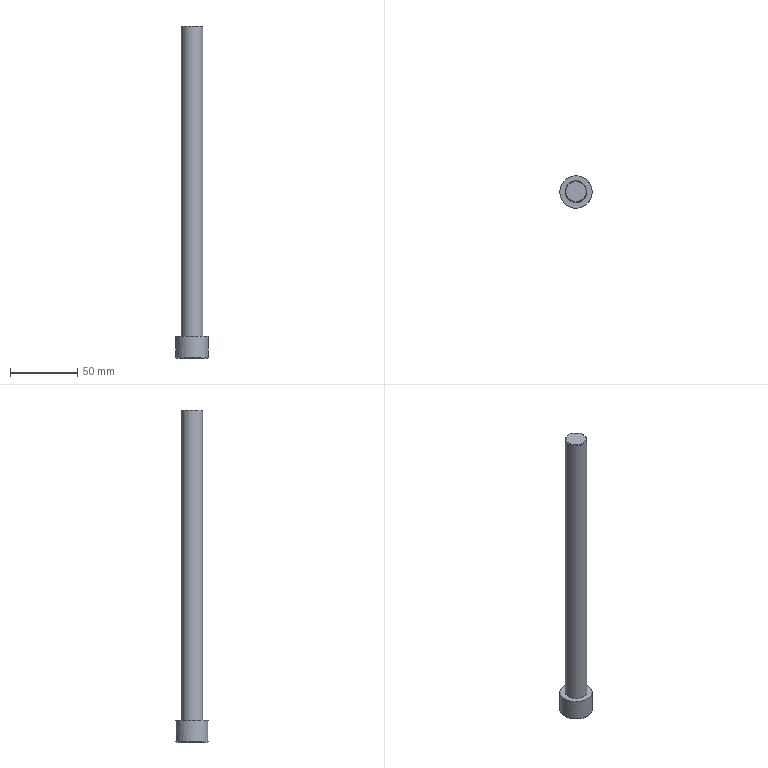Part | NX | features solid 2 | 1 solid | 14 faces | box 24 x 24 x 246 mm | volume 52114 mm3 | plane 10 | cylinder 2 | torus 1 | cone 1 | commonest cylinder face diameters 16 x1 24 x1
STEP:
#1=CARTESIAN_POINT('',(169.041,134.,-412.5));
#2=VERTEX_POINT('',#1);
#3=CARTESIAN_POINT('',(173.083,127.,-412.5));
#4=VERTEX_POINT('',#3);
#5=CARTESIAN_POINT('',(169.041,134.,-412.5));
#6=DIRECTION('',(0.5,-0.866,0.));
#7=VECTOR('',#6,1000.);
#8=LINE('',#5,#7);
#9=EDGE_CURVE('',#2,#4,#8,.T.);
#10=ORIENTED_EDGE('',*,*,#9,.F.);
#11=CARTESIAN_POINT('',(160.959,134.,-412.5));
#12=VERTEX_POINT('',#11);
#13=CARTESIAN_POINT('',(160.959,134.,-412.5));
#14=DIRECTION('',(1.,0.,0.));
#15=VECTOR('',#14,1000.);
#16=LINE('',#13,#15);
#17=EDGE_CURVE('',#12,#2,#16,.T.);
#18=ORIENTED_EDGE('',*,*,#17,.F.);
#19=CARTESIAN_POINT('',(156.917,127.,-412.5));
#20=VERTEX_POINT('',#19);
#21=CARTESIAN_POINT('',(156.917,127.,-412.5));
#22=DIRECTION('',(0.5,0.866,0.));
#23=VECTOR('',#22,1000.);
#24=LINE('',#21,#23);
#25=EDGE_CURVE('',#20,#12,#24,.T.);
#26=ORIENTED_EDGE('',*,*,#25,.F.);
#27=CARTESIAN_POINT('',(160.959,120.,-412.5));
#28=VERTEX_POINT('',#27);
#29=CARTESIAN_POINT('',(160.959,120.,-412.5));
#30=DIRECTION('',(-0.5,0.866,0.));
#31=VECTOR('',#30,1000.);
#32=LINE('',#29,#31);
#33=EDGE_CURVE('',#28,#20,#32,.T.);
#34=ORIENTED_EDGE('',*,*,#33,.F.);
#35=CARTESIAN_POINT('',(169.041,120.,-412.5));
#36=VERTEX_POINT('',#35);
#37=CARTESIAN_POINT('',(169.041,120.,-412.5));
#38=DIRECTION('',(-1.,0.,0.));
#39=VECTOR('',#38,1000.);
#40=LINE('',#37,#39);
#41=EDGE_CURVE('',#36,#28,#40,.T.);
#42=ORIENTED_EDGE('',*,*,#41,.F.);
#43=CARTESIAN_POINT('',(173.083,127.,-412.5));
#44=DIRECTION('',(-0.5,-0.866,0.));
#45=VECTOR('',#44,1000.);
#46=LINE('',#43,#45);
#47=EDGE_CURVE('',#4,#36,#46,.T.);
#48=ORIENTED_EDGE('',*,*,#47,.F.);
#49=EDGE_LOOP('',(#10,#18,#26,#34,#42,#48));
#50=FACE_BOUND('',#49,.T.);
#51=CARTESIAN_POINT('',(165.,138.5,-412.5));
#52=VERTEX_POINT('',#51);
#53=CARTESIAN_POINT('',(165.,127.,-412.5));
#54=DIRECTION('',(0.,0.,-1.));
#55=DIRECTION('',(0.,1.,0.));
#56=AXIS2_PLACEMENT_3D('',#53,#54,#55);
#57=CIRCLE('',#56,11.5);
#58=EDGE_CURVE('',#52,#52,#57,.T.);
#59=ORIENTED_EDGE('',*,*,#58,.T.);
#60=EDGE_LOOP('',(#59));
#61=FACE_BOUND('',#60,.T.);
#62=CARTESIAN_POINT('',(165.,127.,-412.5));
#63=DIRECTION('',(0.,0.,-1.));
#64=DIRECTION('',(0.,1.,0.));
#65=AXIS2_PLACEMENT_3D('',#62,#63,#64);
#66=PLANE('',#65);
#67=ADVANCED_FACE('',(#50,#61),#66,.T.);
#68=CARTESIAN_POINT('',(165.,119.,-396.5));
#69=VERTEX_POINT('',#68);
#70=CARTESIAN_POINT('',(165.,127.,-396.5));
#71=DIRECTION('',(0.,0.,1.));
#72=DIRECTION('',(0.,-1.,0.));
#73=AXIS2_PLACEMENT_3D('',#70,#71,#72);
#74=CIRCLE('',#73,8.);
#75=EDGE_CURVE('',#69,#69,#74,.T.);
#76=ORIENTED_EDGE('',*,*,#75,.F.);
#77=EDGE_LOOP('',(#76));
#78=FACE_BOUND('',#77,.T.);
#79=CARTESIAN_POINT('',(177.,127.,-396.5));
#80=VERTEX_POINT('',#79);
#81=CARTESIAN_POINT('',(165.,127.,-396.5));
#82=DIRECTION('',(0.,0.,-1.));
#83=DIRECTION('',(1.,0.,0.));
#84=AXIS2_PLACEMENT_3D('',#81,#82,#83);
#85=CIRCLE('',#84,12.);
#86=EDGE_CURVE('',#80,#80,#85,.T.);
#87=ORIENTED_EDGE('',*,*,#86,.F.);
#88=EDGE_LOOP('',(#87));
#89=FACE_BOUND('',#88,.T.);
#90=CARTESIAN_POINT('',(165.,127.,-396.5));
#91=DIRECTION('',(0.,0.,1.));
#92=DIRECTION('',(0.,-1.,0.));
#93=AXIS2_PLACEMENT_3D('',#90,#91,#92);
#94=PLANE('',#93);
#95=ADVANCED_FACE('',(#78,#89),#94,.T.);
#96=CARTESIAN_POINT('',(165.,139.,-412.));
#97=VERTEX_POINT('',#96);
#98=CARTESIAN_POINT('',(165.,127.,-412.));
#99=DIRECTION('',(0.,0.,-1.));
#100=DIRECTION('',(0.,1.,0.));
#101=AXIS2_PLACEMENT_3D('',#98,#99,#100);
#102=CIRCLE('',#101,12.);
#103=EDGE_CURVE('',#97,#97,#102,.F.);
#104=ORIENTED_EDGE('',*,*,#103,.T.);
#105=EDGE_LOOP('',(#104));
#106=FACE_BOUND('',#105,.T.);
#107=ORIENTED_EDGE('',*,*,#86,.T.);
#108=EDGE_LOOP('',(#107));
#109=FACE_BOUND('',#108,.T.);
#110=CARTESIAN_POINT('',(165.,127.,-396.5));
#111=DIRECTION('',(0.,0.,-1.));
#112=DIRECTION('',(1.,0.,0.));
#113=AXIS2_PLACEMENT_3D('',#110,#111,#112);
#114=CYLINDRICAL_SURFACE('',#113,12.);
#115=ADVANCED_FACE('',(#106,#109),#114,.T.);
#116=ORIENTED_EDGE('',*,*,#58,.F.);
#117=EDGE_LOOP('',(#116));
#118=FACE_BOUND('',#117,.T.);
#119=ORIENTED_EDGE('',*,*,#103,.F.);
#120=EDGE_LOOP('',(#119));
#121=FACE_BOUND('',#120,.T.);
#122=CARTESIAN_POINT('',(165.,127.,-412.));
#123=DIRECTION('',(0.,0.,-1.));
#124=DIRECTION('',(0.,1.,0.));
#125=AXIS2_PLACEMENT_3D('',#122,#123,#124);
#126=TOROIDAL_SURFACE('',#125,11.5,0.5);
#127=ADVANCED_FACE('',(#118,#121),#126,.T.);
#128=CARTESIAN_POINT('',(165.,119.5,-166.5));
#129=VERTEX_POINT('',#128);
#130=CARTESIAN_POINT('',(165.,127.,-166.5));
#131=DIRECTION('',(0.,0.,1.));
#132=DIRECTION('',(0.,-1.,0.));
#133=AXIS2_PLACEMENT_3D('',#130,#131,#132);
#134=CIRCLE('',#133,7.5);
#135=EDGE_CURVE('',#129,#129,#134,.T.);
#136=ORIENTED_EDGE('',*,*,#135,.T.);
#137=EDGE_LOOP('',(#136));
#138=FACE_BOUND('',#137,.T.);
#139=CARTESIAN_POINT('',(165.,127.,-166.5));
#140=DIRECTION('',(0.,0.,1.));
#141=DIRECTION('',(0.,-1.,0.));
#142=AXIS2_PLACEMENT_3D('',#139,#140,#141);
#143=PLANE('',#142);
#144=ADVANCED_FACE('',(#138),#143,.T.);
#145=CARTESIAN_POINT('',(173.,127.,-167.));
#146=VERTEX_POINT('',#145);
#147=CARTESIAN_POINT('',(165.,127.,-167.));
#148=DIRECTION('',(0.,0.,1.));
#149=DIRECTION('',(1.,0.,0.));
#150=AXIS2_PLACEMENT_3D('',#147,#148,#149);
#151=CIRCLE('',#150,8.);
#152=EDGE_CURVE('',#146,#146,#151,.F.);
#153=ORIENTED_EDGE('',*,*,#152,.T.);
#154=EDGE_LOOP('',(#153));
#155=FACE_BOUND('',#154,.T.);
#156=ORIENTED_EDGE('',*,*,#75,.T.);
#157=EDGE_LOOP('',(#156));
#158=FACE_BOUND('',#157,.T.);
#159=CARTESIAN_POINT('',(165.,127.,-166.5));
#160=DIRECTION('',(0.,0.,-1.));
#161=DIRECTION('',(1.,0.,0.));
#162=AXIS2_PLACEMENT_3D('',#159,#160,#161);
#163=CYLINDRICAL_SURFACE('',#162,8.);
#164=ADVANCED_FACE('',(#155,#158),#163,.T.);
#165=ORIENTED_EDGE('',*,*,#135,.F.);
#166=EDGE_LOOP('',(#165));
#167=FACE_BOUND('',#166,.T.);
#168=ORIENTED_EDGE('',*,*,#152,.F.);
#169=EDGE_LOOP('',(#168));
#170=FACE_BOUND('',#169,.T.);
#171=CARTESIAN_POINT('',(165.,127.,-167.));
#172=DIRECTION('',(0.,0.,-1.));
#173=DIRECTION('',(-1.,0.,0.));
#174=AXIS2_PLACEMENT_3D('',#171,#172,#173);
#175=CONICAL_SURFACE('',#174,8.,0.7854);
#176=ADVANCED_FACE('',(#167,#170),#175,.T.);
#177=ORIENTED_EDGE('',*,*,#9,.T.);
#178=CARTESIAN_POINT('',(173.083,127.,-404.5));
#179=VERTEX_POINT('',#178);
#180=CARTESIAN_POINT('',(173.083,127.,-404.5));
#181=DIRECTION('',(0.,0.,-1.));
#182=VECTOR('',#181,1000.);
#183=LINE('',#180,#182);
#184=EDGE_CURVE('',#179,#4,#183,.T.);
#185=ORIENTED_EDGE('',*,*,#184,.F.);
#186=CARTESIAN_POINT('',(169.041,134.,-404.5));
#187=VERTEX_POINT('',#186);
#188=CARTESIAN_POINT('',(169.041,134.,-404.5));
#189=DIRECTION('',(0.5,-0.866,0.));
#190=VECTOR('',#189,1000.);
#191=LINE('',#188,#190);
#192=EDGE_CURVE('',#187,#179,#191,.T.);
#193=ORIENTED_EDGE('',*,*,#192,.F.);
#194=CARTESIAN_POINT('',(169.041,134.,-404.5));
#195=DIRECTION('',(0.,0.,-1.));
#196=VECTOR('',#195,1000.);
#197=LINE('',#194,#196);
#198=EDGE_CURVE('',#187,#2,#197,.T.);
#199=ORIENTED_EDGE('',*,*,#198,.T.);
#200=EDGE_LOOP('',(#177,#185,#193,#199));
#201=FACE_BOUND('',#200,.T.);
#202=CARTESIAN_POINT('',(171.062,130.5,-408.5));
#203=DIRECTION('',(0.866,0.5,0.));
#204=DIRECTION('',(-0.5,0.866,0.));
#205=AXIS2_PLACEMENT_3D('',#202,#203,#204);
#206=PLANE('',#205);
#207=ADVANCED_FACE('',(#201),#206,.F.);
#208=ORIENTED_EDGE('',*,*,#17,.T.);
#209=ORIENTED_EDGE('',*,*,#198,.F.);
#210=CARTESIAN_POINT('',(160.959,134.,-404.5));
#211=VERTEX_POINT('',#210);
#212=CARTESIAN_POINT('',(160.959,134.,-404.5));
#213=DIRECTION('',(1.,0.,0.));
#214=VECTOR('',#213,1000.);
#215=LINE('',#212,#214);
#216=EDGE_CURVE('',#211,#187,#215,.T.);
#217=ORIENTED_EDGE('',*,*,#216,.F.);
#218=CARTESIAN_POINT('',(160.959,134.,-404.5));
#219=DIRECTION('',(0.,0.,-1.));
#220=VECTOR('',#219,1000.);
#221=LINE('',#218,#220);
#222=EDGE_CURVE('',#211,#12,#221,.T.);
#223=ORIENTED_EDGE('',*,*,#222,.T.);
#224=EDGE_LOOP('',(#208,#209,#217,#223));
#225=FACE_BOUND('',#224,.T.);
#226=CARTESIAN_POINT('',(165.,134.,-408.5));
#227=DIRECTION('',(0.,1.,0.));
#228=DIRECTION('',(0.,0.,1.));
#229=AXIS2_PLACEMENT_3D('',#226,#227,#228);
#230=PLANE('',#229);
#231=ADVANCED_FACE('',(#225),#230,.F.);
#232=ORIENTED_EDGE('',*,*,#25,.T.);
#233=ORIENTED_EDGE('',*,*,#222,.F.);
#234=CARTESIAN_POINT('',(156.917,127.,-404.5));
#235=VERTEX_POINT('',#234);
#236=CARTESIAN_POINT('',(156.917,127.,-404.5));
#237=DIRECTION('',(0.5,0.866,0.));
#238=VECTOR('',#237,1000.);
#239=LINE('',#236,#238);
#240=EDGE_CURVE('',#235,#211,#239,.T.);
#241=ORIENTED_EDGE('',*,*,#240,.F.);
#242=CARTESIAN_POINT('',(156.917,127.,-404.5));
#243=DIRECTION('',(0.,0.,-1.));
#244=VECTOR('',#243,1000.);
#245=LINE('',#242,#244);
#246=EDGE_CURVE('',#235,#20,#245,.T.);
#247=ORIENTED_EDGE('',*,*,#246,.T.);
#248=EDGE_LOOP('',(#232,#233,#241,#247));
#249=FACE_BOUND('',#248,.T.);
#250=CARTESIAN_POINT('',(158.938,130.5,-408.5));
#251=DIRECTION('',(-0.866,0.5,0.));
#252=DIRECTION('',(-0.5,-0.866,0.));
#253=AXIS2_PLACEMENT_3D('',#250,#251,#252);
#254=PLANE('',#253);
#255=ADVANCED_FACE('',(#249),#254,.F.);
#256=ORIENTED_EDGE('',*,*,#33,.T.);
#257=ORIENTED_EDGE('',*,*,#246,.F.);
#258=CARTESIAN_POINT('',(160.959,120.,-404.5));
#259=VERTEX_POINT('',#258);
#260=CARTESIAN_POINT('',(160.959,120.,-404.5));
#261=DIRECTION('',(-0.5,0.866,0.));
#262=VECTOR('',#261,1000.);
#263=LINE('',#260,#262);
#264=EDGE_CURVE('',#259,#235,#263,.T.);
#265=ORIENTED_EDGE('',*,*,#264,.F.);
#266=CARTESIAN_POINT('',(160.959,120.,-404.5));
#267=DIRECTION('',(0.,0.,-1.));
#268=VECTOR('',#267,1000.);
#269=LINE('',#266,#268);
#270=EDGE_CURVE('',#259,#28,#269,.T.);
#271=ORIENTED_EDGE('',*,*,#270,.T.);
#272=EDGE_LOOP('',(#256,#257,#265,#271));
#273=FACE_BOUND('',#272,.T.);
#274=CARTESIAN_POINT('',(158.938,123.5,-408.5));
#275=DIRECTION('',(-0.866,-0.5,0.));
#276=DIRECTION('',(0.5,-0.866,0.));
#277=AXIS2_PLACEMENT_3D('',#274,#275,#276);
#278=PLANE('',#277);
#279=ADVANCED_FACE('',(#273),#278,.F.);
#280=ORIENTED_EDGE('',*,*,#41,.T.);
#281=ORIENTED_EDGE('',*,*,#270,.F.);
#282=CARTESIAN_POINT('',(169.041,120.,-404.5));
#283=VERTEX_POINT('',#282);
#284=CARTESIAN_POINT('',(169.041,120.,-404.5));
#285=DIRECTION('',(-1.,0.,0.));
#286=VECTOR('',#285,1000.);
#287=LINE('',#284,#286);
#288=EDGE_CURVE('',#283,#259,#287,.T.);
#289=ORIENTED_EDGE('',*,*,#288,.F.);
#290=CARTESIAN_POINT('',(169.041,120.,-404.5));
#291=DIRECTION('',(0.,0.,-1.));
#292=VECTOR('',#291,1000.);
#293=LINE('',#290,#292);
#294=EDGE_CURVE('',#283,#36,#293,.T.);
#295=ORIENTED_EDGE('',*,*,#294,.T.);
#296=EDGE_LOOP('',(#280,#281,#289,#295));
#297=FACE_BOUND('',#296,.T.);
#298=CARTESIAN_POINT('',(165.,120.,-408.5));
#299=DIRECTION('',(0.,-1.,0.));
#300=DIRECTION('',(0.,0.,-1.));
#301=AXIS2_PLACEMENT_3D('',#298,#299,#300);
#302=PLANE('',#301);
#303=ADVANCED_FACE('',(#297),#302,.F.);
#304=ORIENTED_EDGE('',*,*,#47,.T.);
#305=ORIENTED_EDGE('',*,*,#294,.F.);
#306=CARTESIAN_POINT('',(173.083,127.,-404.5));
#307=DIRECTION('',(-0.5,-0.866,0.));
#308=VECTOR('',#307,1000.);
#309=LINE('',#306,#308);
#310=EDGE_CURVE('',#179,#283,#309,.T.);
#311=ORIENTED_EDGE('',*,*,#310,.F.);
#312=ORIENTED_EDGE('',*,*,#184,.T.);
#313=EDGE_LOOP('',(#304,#305,#311,#312));
#314=FACE_BOUND('',#313,.T.);
#315=CARTESIAN_POINT('',(171.062,123.5,-408.5));
#316=DIRECTION('',(0.866,-0.5,0.));
#317=DIRECTION('',(0.5,0.866,0.));
#318=AXIS2_PLACEMENT_3D('',#315,#316,#317);
#319=PLANE('',#318);
#320=ADVANCED_FACE('',(#314),#319,.F.);
#321=ORIENTED_EDGE('',*,*,#310,.T.);
#322=ORIENTED_EDGE('',*,*,#288,.T.);
#323=ORIENTED_EDGE('',*,*,#264,.T.);
#324=ORIENTED_EDGE('',*,*,#240,.T.);
#325=ORIENTED_EDGE('',*,*,#216,.T.);
#326=ORIENTED_EDGE('',*,*,#192,.T.);
#327=EDGE_LOOP('',(#321,#322,#323,#324,#325,#326));
#328=FACE_BOUND('',#327,.T.);
#329=CARTESIAN_POINT('',(165.,127.,-404.5));
#330=DIRECTION('',(0.,0.,1.));
#331=DIRECTION('',(0.,-1.,0.));
#332=AXIS2_PLACEMENT_3D('',#329,#330,#331);
#333=PLANE('',#332);
#334=ADVANCED_FACE('',(#328),#333,.F.);
#335=CLOSED_SHELL('',(#67,#95,#115,#127,#144,#164,#176,#207,#231,#255,#279,#303,#320,#334));
#336=MANIFOLD_SOLID_BREP('',#335);
#337=(LENGTH_UNIT()NAMED_UNIT(*)SI_UNIT(.MILLI.,.METRE.));
#338=UNCERTAINTY_MEASURE_WITH_UNIT(LENGTH_MEASURE(0.00001),#337,'','');
#339=(NAMED_UNIT(*)PLANE_ANGLE_UNIT()SI_UNIT($,.RADIAN.));
#340=(NAMED_UNIT(*)SI_UNIT($,.STERADIAN.)SOLID_ANGLE_UNIT());
#341=(GEOMETRIC_REPRESENTATION_CONTEXT(3)GLOBAL_UNCERTAINTY_ASSIGNED_CONTEXT((#338))GLOBAL_UNIT_ASSIGNED_CONTEXT((#337,#339,#340))REPRESENTATION_CONTEXT('',''));
#342=ADVANCED_BREP_SHAPE_REPRESENTATION('',(#336),#341);